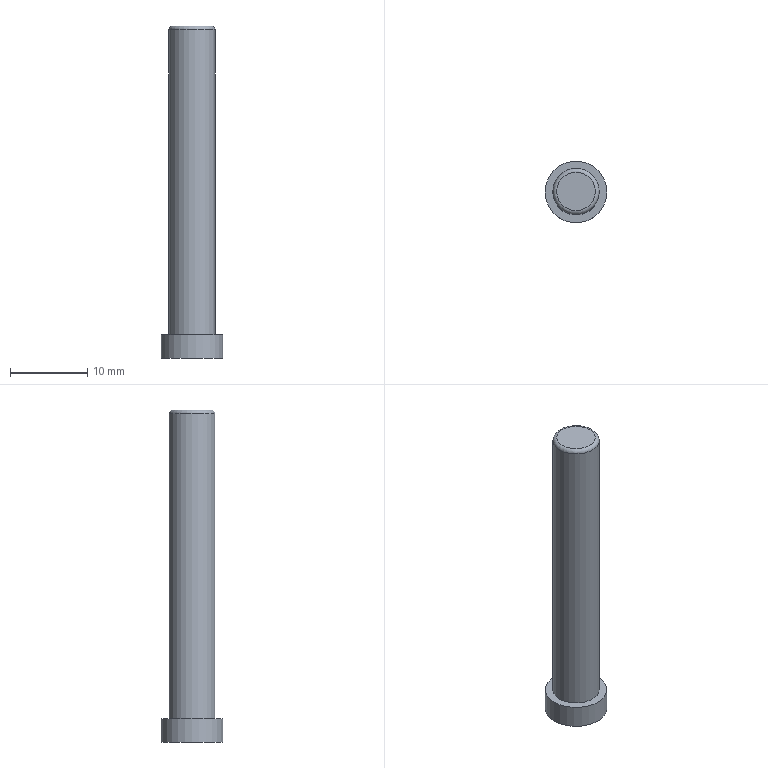Part | STEP file | lll_id4162_x_t | 1 solid | 6 faces | box 8 x 8 x 43 mm | volume 1281 mm3 | plane 3 | cylinder 2 | torus 1 | commonest cylinder face diameters 6 x1 8 x1
STEP:
#1=CARTESIAN_POINT('',(3859.,-51.75,4.5));
#2=VERTEX_POINT('',#1);
#3=CARTESIAN_POINT('',(3862.,-51.75,4.5));
#4=DIRECTION('',(0.,0.,1.));
#5=DIRECTION('',(-1.,0.,0.));
#6=AXIS2_PLACEMENT_3D('',#3,#4,#5);
#7=CIRCLE('',#6,3.);
#8=EDGE_CURVE('',#2,#2,#7,.T.);
#9=ORIENTED_EDGE('',*,*,#8,.F.);
#10=EDGE_LOOP('',(#9));
#11=FACE_BOUND('',#10,.T.);
#12=CARTESIAN_POINT('',(3859.,-51.75,-35.));
#13=VERTEX_POINT('',#12);
#14=CARTESIAN_POINT('',(3862.,-51.75,-35.));
#15=DIRECTION('',(0.,0.,-1.));
#16=DIRECTION('',(-1.,0.,0.));
#17=AXIS2_PLACEMENT_3D('',#14,#15,#16);
#18=CIRCLE('',#17,3.);
#19=EDGE_CURVE('',#13,#13,#18,.T.);
#20=ORIENTED_EDGE('',*,*,#19,.F.);
#21=EDGE_LOOP('',(#20));
#22=FACE_BOUND('',#21,.T.);
#23=CARTESIAN_POINT('',(3862.,-51.75,22.259));
#24=DIRECTION('',(0.,0.,-1.));
#25=DIRECTION('',(0.,-1.,0.));
#26=AXIS2_PLACEMENT_3D('',#23,#24,#25);
#27=CYLINDRICAL_SURFACE('',#26,3.);
#28=ADVANCED_FACE('',(#11,#22),#27,.T.);
#29=CARTESIAN_POINT('',(3859.5,-51.75,5.));
#30=VERTEX_POINT('',#29);
#31=CARTESIAN_POINT('',(3862.,-51.75,5.));
#32=DIRECTION('',(0.,0.,-1.));
#33=DIRECTION('',(-1.,0.,0.));
#34=AXIS2_PLACEMENT_3D('',#31,#32,#33);
#35=CIRCLE('',#34,2.5);
#36=EDGE_CURVE('',#30,#30,#35,.T.);
#37=ORIENTED_EDGE('',*,*,#36,.F.);
#38=EDGE_LOOP('',(#37));
#39=FACE_OUTER_BOUND('',#38,.T.);
#40=CARTESIAN_POINT('',(3685.89,1124.521,5.));
#41=DIRECTION('',(0.,0.,-1.));
#42=DIRECTION('',(0.,-1.,0.));
#43=AXIS2_PLACEMENT_3D('',#40,#41,#42);
#44=PLANE('',#43);
#45=ADVANCED_FACE('',(#39),#44,.F.);
#46=ORIENTED_EDGE('',*,*,#8,.T.);
#47=EDGE_LOOP('',(#46));
#48=FACE_BOUND('',#47,.T.);
#49=ORIENTED_EDGE('',*,*,#36,.T.);
#50=EDGE_LOOP('',(#49));
#51=FACE_BOUND('',#50,.T.);
#52=CARTESIAN_POINT('',(3862.,-51.75,4.5));
#53=DIRECTION('',(0.,0.,-1.));
#54=DIRECTION('',(-1.,0.,0.));
#55=AXIS2_PLACEMENT_3D('',#52,#53,#54);
#56=TOROIDAL_SURFACE('',#55,2.5,0.5);
#57=ADVANCED_FACE('',(#48,#51),#56,.T.);
#58=CARTESIAN_POINT('',(3858.,-51.75,-35.));
#59=VERTEX_POINT('',#58);
#60=CARTESIAN_POINT('',(3862.,-51.75,-35.));
#61=DIRECTION('',(0.,0.,-1.));
#62=DIRECTION('',(-1.,0.,0.));
#63=AXIS2_PLACEMENT_3D('',#60,#61,#62);
#64=CIRCLE('',#63,4.);
#65=EDGE_CURVE('',#59,#59,#64,.T.);
#66=ORIENTED_EDGE('',*,*,#65,.F.);
#67=EDGE_LOOP('',(#66));
#68=FACE_BOUND('',#67,.T.);
#69=ORIENTED_EDGE('',*,*,#19,.T.);
#70=EDGE_LOOP('',(#69));
#71=FACE_BOUND('',#70,.T.);
#72=CARTESIAN_POINT('',(3685.89,1124.521,-35.));
#73=DIRECTION('',(0.,0.,-1.));
#74=DIRECTION('',(0.,-1.,0.));
#75=AXIS2_PLACEMENT_3D('',#72,#73,#74);
#76=PLANE('',#75);
#77=ADVANCED_FACE('',(#68,#71),#76,.F.);
#78=CARTESIAN_POINT('',(3858.,-51.75,-38.));
#79=VERTEX_POINT('',#78);
#80=CARTESIAN_POINT('',(3862.,-51.75,-38.));
#81=DIRECTION('',(0.,0.,-1.));
#82=DIRECTION('',(-1.,0.,0.));
#83=AXIS2_PLACEMENT_3D('',#80,#81,#82);
#84=CIRCLE('',#83,4.);
#85=EDGE_CURVE('',#79,#79,#84,.T.);
#86=ORIENTED_EDGE('',*,*,#85,.F.);
#87=EDGE_LOOP('',(#86));
#88=FACE_BOUND('',#87,.T.);
#89=ORIENTED_EDGE('',*,*,#65,.T.);
#90=EDGE_LOOP('',(#89));
#91=FACE_BOUND('',#90,.T.);
#92=CARTESIAN_POINT('',(3862.,-51.75,-53.741));
#93=DIRECTION('',(0.,0.,1.));
#94=DIRECTION('',(0.,1.,0.));
#95=AXIS2_PLACEMENT_3D('',#92,#93,#94);
#96=CYLINDRICAL_SURFACE('',#95,4.);
#97=ADVANCED_FACE('',(#88,#91),#96,.T.);
#98=ORIENTED_EDGE('',*,*,#85,.T.);
#99=EDGE_LOOP('',(#98));
#100=FACE_OUTER_BOUND('',#99,.T.);
#101=CARTESIAN_POINT('',(3685.89,1124.521,-38.));
#102=DIRECTION('',(0.,0.,-1.));
#103=DIRECTION('',(0.,-1.,0.));
#104=AXIS2_PLACEMENT_3D('',#101,#102,#103);
#105=PLANE('',#104);
#106=ADVANCED_FACE('',(#100),#105,.T.);
#107=CLOSED_SHELL('',(#28,#45,#57,#77,#97,#106));
#108=MANIFOLD_SOLID_BREP('',#107);
#109=(LENGTH_UNIT()NAMED_UNIT(*)SI_UNIT(.MILLI.,.METRE.));
#110=UNCERTAINTY_MEASURE_WITH_UNIT(LENGTH_MEASURE(0.00002),#109,'','');
#111=(NAMED_UNIT(*)PLANE_ANGLE_UNIT()SI_UNIT($,.RADIAN.));
#112=PLANE_ANGLE_MEASURE_WITH_UNIT(PLANE_ANGLE_MEASURE(0.01745),#111);
#113=DIMENSIONAL_EXPONENTS(0.,0.,0.,0.,0.,0.,0.);
#114=(CONVERSION_BASED_UNIT('DEGREE',#112)NAMED_UNIT(#113)PLANE_ANGLE_UNIT());
#115=(NAMED_UNIT(*)SI_UNIT($,.STERADIAN.)SOLID_ANGLE_UNIT());
#116=(GEOMETRIC_REPRESENTATION_CONTEXT(3)GLOBAL_UNCERTAINTY_ASSIGNED_CONTEXT((#110))GLOBAL_UNIT_ASSIGNED_CONTEXT((#109,#114,#115))REPRESENTATION_CONTEXT('',''));
#117=ADVANCED_BREP_SHAPE_REPRESENTATION('',(#108),#116);